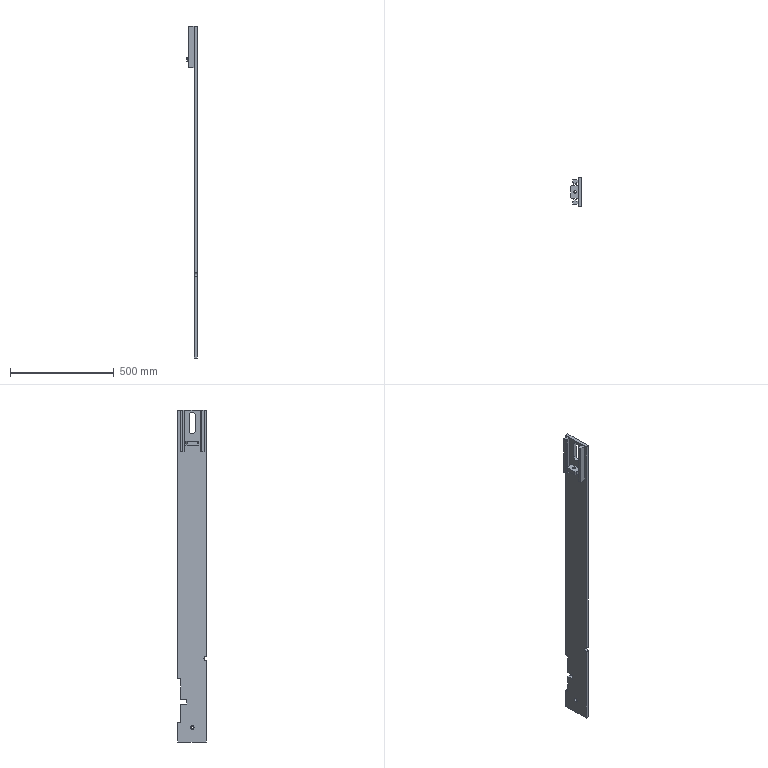Part | STEP file | PN_0020 | 3 solids | 54 faces | box 50 x 139 x 1600 mm | volume 3436426 mm3 | plane 45 | cylinder 9 | commonest cylinder face diameters 11 x2 12 x2 18 x2 30 x2 20 x1